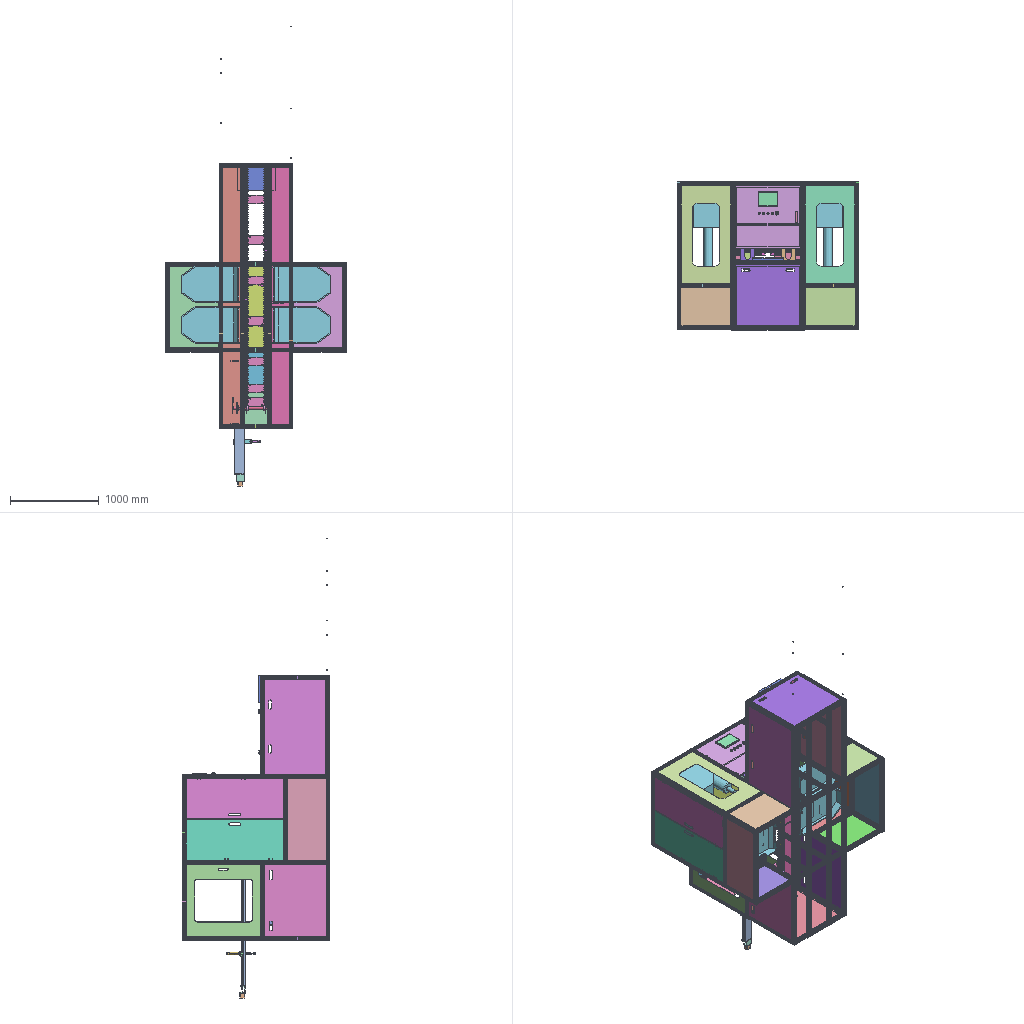Assembly | STEP file | 102 different items | 1017 placed | box 2053 x 1672 x 5196 mm
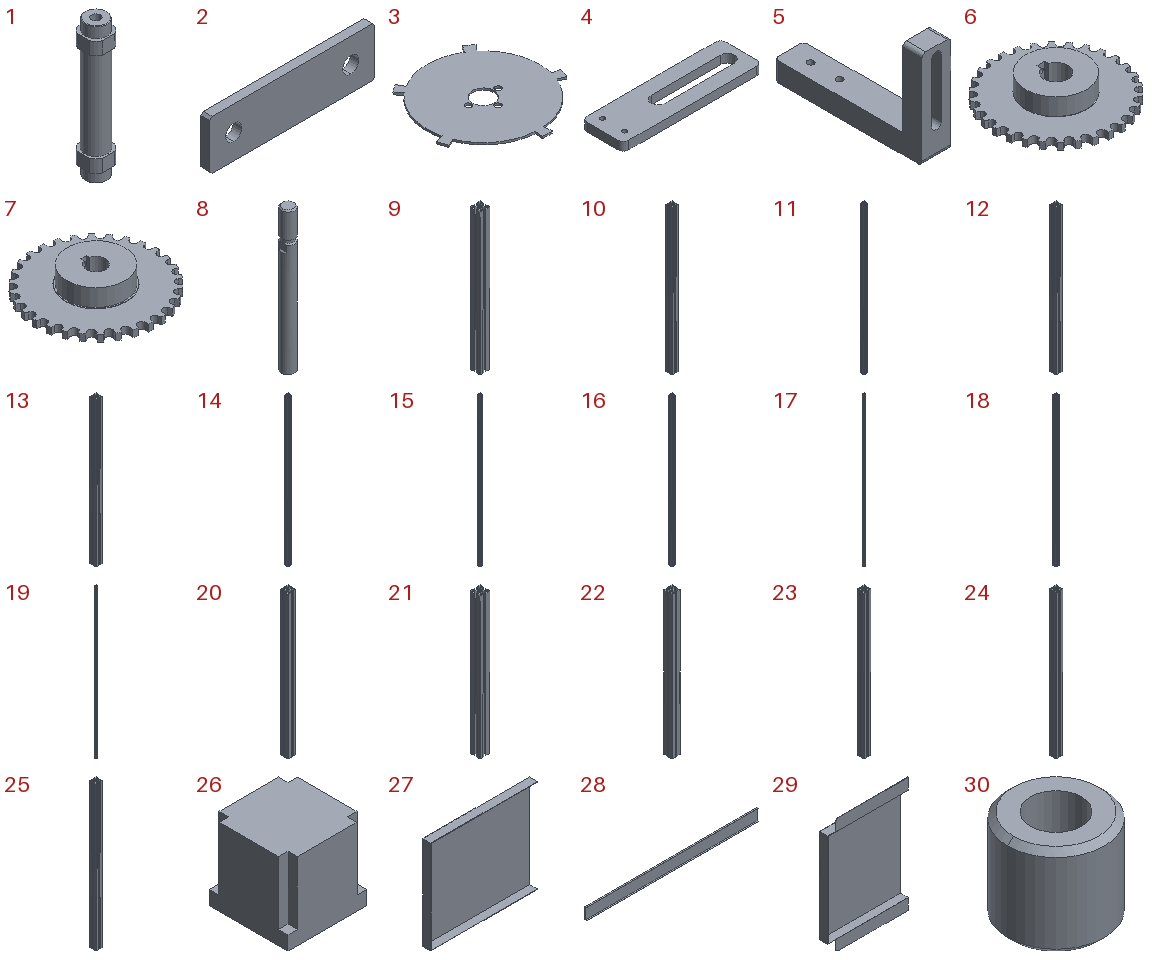Parts list (item | name | quantity | parent item | size | volume):
1 | 1-2 | x1 | in A_CM2B25-75(0)气缸-2 | 30 x 30 x 163 mm | 89864 mm3
2 | 1004-2001-0021_1004-2001-0021_1-2 | x2 | - | 134 x 7 x 40 mm | 35606 mm3
3 | 1004-2001-0084_1004-2001-0084_1-2 | x1 | - | 126.387 x 122 x 2 mm | 20227 mm3
4 | 1004-2001-0085_1004-2001-0085_1-2 | x1 | - | 50 x 15 x 3 mm | 1794 mm3
5 | 1004-2001-0086-1_1004-2001-0086-2 | x1 | - | 15 x 76 x 50 mm | 15485 mm3
6 | 1004-2001-0088_1004-2001-0088_1-2 | x2 | - | 128 x 127.688 x 25 mm | 125433 mm3
7 | 1004-2001-0089_1004-2001-0089_1-2 | x1 | - | 128 x 127.688 x 25 mm | 124903 mm3
8 | 2-2 | x1 | in A_CM2B25-75(0)气缸-2 | 10 x 10 x 108 mm | 8348 mm3
9 | 40-570-2 | x2 | in PN_0001_ASM-2 | 40 x 40 x 570 mm | 299104 mm3
10 | 40C-2 | x1 | in JZ_ASM_1_ASM-2 | 40 x 40 x 930 mm | 488011 mm3
11 | 40D-2 | x1 | in JZ_ASM_1_ASM-2 | 40 x 40 x 1670 mm | 876321 mm3
12 | 40T-2 | x1 | in JZ_ASM_1_ASM-2 | 40 x 40 x 930 mm | 488011 mm3
13 | 40U-2 | x1 | in JZ_ASM_1_ASM-2 | 40 x 40 x 930 mm | 488011 mm3
14 | 40V-2 | x1 | in JZ_ASM_1_ASM-2 | 40 x 40 x 1670 mm | 876321 mm3
15 | 40_40_1350_1-2 | x4 | in JZ_ASM_1_ASM-2 | 40 x 40 x 1970 mm | 1033744 mm3
16 | 40_40_1590_1-2 | x2 | in JZ_ASM_1_ASM-2 | 40 x 40 x 1670 mm | 876321 mm3
17 | 40_40_2730_1-2 | x2 | in JZ_ASM_1_ASM-2 | 40 x 40 x 2990 mm | 1568982 mm3
18 | 40_40_3240_1-2 | x2 | in JZ_ASM_1_ASM-2 | 40 x 40 x 1875 mm | 983893 mm3
19 | 40_40_4640_1-2 | x6 | in JZ_ASM_1_ASM-2 | 40 x 40 x 2989 mm | 1568656 mm3
20 | 40_40_470_1-2 | x2 | in JZ_ASM_1_ASM-2 | 40 x 40 x 750 mm | 393557 mm3
21 | 40_40_570-2 | x2 | in PN_0001_ASM-2 | 40 x 40 x 570 mm | 299104 mm3
22 | 40_40_700_1-2 | x14 | in JZ_ASM_1_ASM-2 | 40 x 40 x 700 mm | 367320 mm3
23 | 40_40_750_1-2 | x5 | in JZ_ASM_1_ASM-2 | 40 x 40 x 830 mm | 435537 mm3
24 | 40_40_850_1-2 | x6 | in JZ_ASM_1_ASM-2 | 40 x 40 x 850 mm | 446032 mm3
25 | 40_40_930_1-2 | x3 | in JZ_ASM_1_ASM-2 | 40 x 40 x 930 mm | 488011 mm3
26 | 57-3260步进马达-2 | x1 | in PN_0001_ASM-2 | 56 x 56 x 77.6 mm | 165142 mm3
27 | B-BAN1_1-2 | x1 | in PN_0001_ASM-2 | 400 x 30 x 350 mm | 259034 mm3
28 | B-BAN2_1-2 | x1 | in PN_0001_ASM-2 | 2950 x 30 x 200 mm | 1137225 mm3
29 | B-BAN5_1-2 | x1 | in PN_0001_ASM-2 | 300 x 30 x 430 mm | 230320 mm3
30 | CHAIN-01_1_02LT_1-2 | x220 | in TUOLIETIAO_ASM_1_ASM-2 | 8.5 x 8.5 x 8 mm | 320.312 mm3
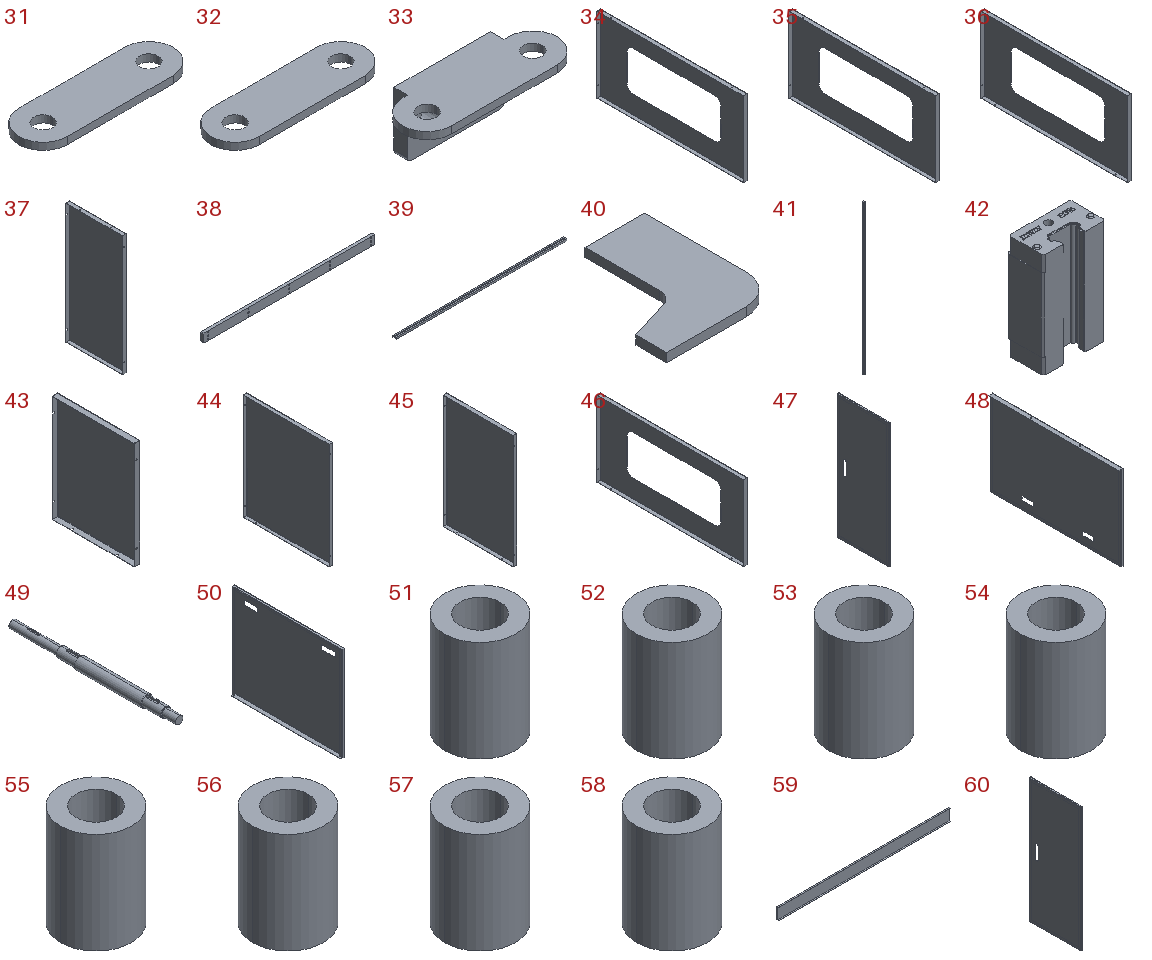31 | CHAIN-02_1_02LT_1-2 | x220 | in TUOLIETIAO_ASM_1_ASM-2 | 37.1 x 11.7 x 1.7 mm | 633.904 mm3
32 | CHAIN-03_1_02LT_1-2 | x216 | in TUOLIETIAO_ASM_1_ASM-2 | 37.1 x 11.7 x 1.7 mm | 633.904 mm3
33 | CHAIN-04_1_02LT_1-2 | x108 | in TUOLIETIAO_ASM_1_ASM-2 | 37.1 x 14.95 x 14.1 mm | 1597 mm3
34 | CHAME-2 | x1 | in PN_0001_ASM-2 | 30 x 1108 x 568 mm | 765086 mm3
35 | CHAME3-2 | x1 | in PN_0001_ASM-2 | 30 x 1108 x 568 mm | 765086 mm3
36 | CHME2-2 | x1 | in PN_0001_ASM-2 | 30 x 1108 x 568 mm | 765102 mm3
37 | CSD4-2 | x1 | in PN_0001_ASM-2 | 30 x 438 x 928 mm | 721285 mm3
38 | DAOLIECHAO-BAN_1-2 | x2 | in LIANTIAO_ASM_1_ASM-2 | 800 x 12 x 40 mm | 378698 mm3
39 | DAOLIECHAO_1-2 | x2 | in LIANTIAO_ASM_1_ASM-2 | 1861 x 40 x 20 mm | 1235153 mm3
40 | Discharge manipulator bracket.SLDASM-2 (subassembly) | x2 | in PN_0001_ASM-2 | 147.814 x 177.869 x 12 mm | 209292 mm3
41 | EG15_RAIL-2 | x1 | in EGH15CA导轨-2 | 15 x 12.5 x 1282 mm | 208724 mm3
42 | EGH15CA_BLOCK-2 | x1 | in EGH15CA导轨-2 | 34 x 19.5 x 57.8 mm | 30496 mm3
43 | FB-3_1-2 | x1 | in PN_0001_ASM-2 | 30 x 438 x 568 mm | 454976 mm3
44 | FB-6_1-2 | x1 | in PN_0001_ASM-2 | 30 x 748 x 923 mm | 1172313 mm3
45 | FB-7_1-2 | x1 | in PN_0001_ASM-2 | 30 x 568 x 923 mm | 908240 mm3
46 | FB-8_1-2 | x1 | in PN_0001_ASM-2 | 30 x 1108 x 568 mm | 765102 mm3
47 | FENGBAN-C-1_1-2 | x2 | in PN_0001_ASM-2 | 15 x 461 x 1106 mm | 897799 mm3
48 | HT-2 | x1 | in PN_0001_ASM-2 | 35 x 1080 x 702 mm | 1298798 mm3
49 | LIELUN30_1-2 | x1 | - | 30 x 432.6 x 30 mm | 218301 mm3
50 | MANIFOLD_SOLID_BREP_304524-2 | x1 | in FENBAN-1_1_ASM-2 | 30 x 816 x 696 mm | 984068 mm3
51 | MANIFOLD_SOLID_BREP_304727-2 | x1 | in FENBAN-1_1_ASM-2 | 7 x 7 x 10 mm | 259.181 mm3
52 | MANIFOLD_SOLID_BREP_304930-2 | x1 | in FENBAN-1_1_ASM-2 | 7 x 7 x 10 mm | 259.181 mm3
53 | MANIFOLD_SOLID_BREP_309818-2 | x8 | in FENBAN-2_1_ASM-2 | 7 x 7 x 10 mm | 259.181 mm3
54 | MANIFOLD_SOLID_BREP_312481-2 | x2 | in FENBAN-3_1_ASM-2 | 7 x 7 x 10 mm | 259.181 mm3
55 | MANIFOLD_SOLID_BREP_312684-2 | x2 | in FENBAN-3_1_ASM-2 | 7 x 7 x 10 mm | 259.181 mm3
56 | MANIFOLD_SOLID_BREP_315330-2 | x2 | in FENBAN-4_1_ASM-2 | 7 x 7 x 10 mm | 259.181 mm3
57 | MANIFOLD_SOLID_BREP_345006-2 | x1 | in FENBAN-5_1_ASM-2 | 7 x 7 x 10 mm | 259.181 mm3
58 | MANIFOLD_SOLID_BREP_345209-2 | x1 | in FENBAN-5_1_ASM-2 | 7 x 7 x 10 mm | 259.181 mm3
59 | MBG-2 | x1 | in PN_0001_ASM-2 | 2950 x 30 x 200 mm | 1137225 mm3
60 | ME4-2 | x1 | in PN_0001_ASM-2 | 15 x 461 x 1106 mm | 897799 mm3
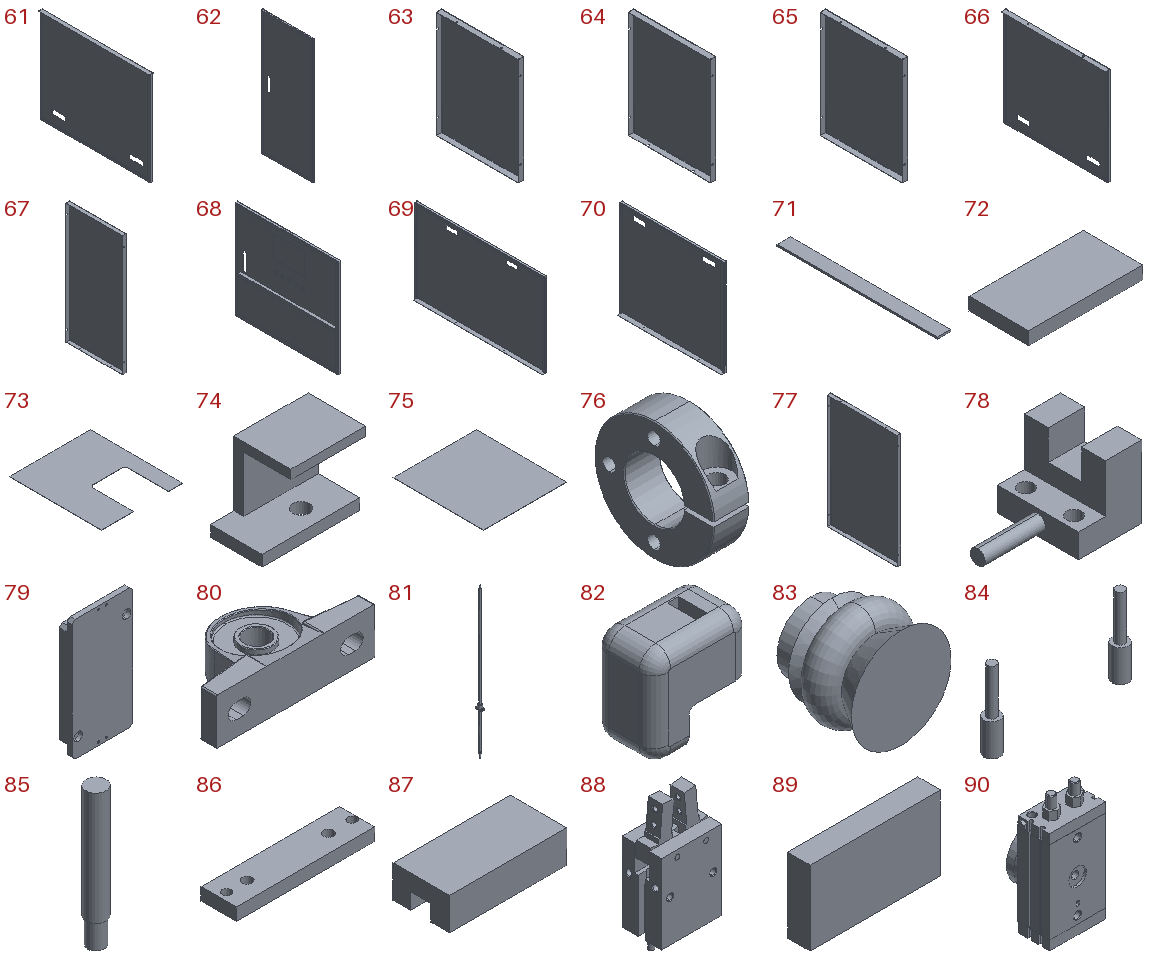61 | MEN-2 | x1 | in PN_0001_ASM-2 | 30 x 816 x 696 mm | 984067 mm3
62 | MEN5-2 | x1 | in PN_0001_ASM-2 | 15 x 461 x 1106 mm | 897799 mm3
63 | MEN7-2 | x1 | in PN_0001_ASM-2 | 30 x 438 x 568 mm | 454976 mm3
64 | MEN87-2 | x1 | in PN_0001_ASM-2 | 30 x 438 x 568 mm | 454976 mm3
65 | MENH-2 | x1 | in PN_0001_ASM-2 | 30 x 438 x 568 mm | 454976 mm3
66 | MRE-2 | x1 | in PN_0001_ASM-2 | 35 x 750 x 702 mm | 920814 mm3
67 | MSBR-1000F-2 | x1 | in PN_0001_ASM-2 | 30 x 438 x 928 mm | 721208 mm3
68 | PRT0544B-HK-005_B9T2-2 | x1 | in PN_0001_ASM-2 | 43.5 x 750 x 710 mm | 1553231 mm3
69 | PRT0544B_HI-00-2 | x1 | in PN_0001_ASM-2 | 35 x 1080 x 702 mm | 1298798 mm3
70 | PRT0544B_HI-003_B-2 | x1 | in PN_0001_ASM-2 | 35 x 750 x 702 mm | 920814 mm3
71 | Part 17 PN_0001_ASM 2 | x1 | in PN_0001_ASM-2 | 106.46 x 1282 x 15 mm | 2047522 mm3
72 | Part 19^PN_0001_ASM-2 | x1 | in PN_0001_ASM-2 | 106.46 x 56 x 12 mm | 71541 mm3
73 | Part 2 PN_0001_ASM 2 | x1 | in PN_0001_ASM-2 | 744 x 848.417 x 2 mm | 1008010 mm3
74 | Part 20 PN_0001_ASM 2 | x1 | in PN_0001_ASM-2 | 106.46 x 62.346 x 82.377 mm | 171045 mm3
75 | Part 3 PN_0001_ASM 2 | x1 | in PN_0001_ASM-2 | 751.5 x 821.5 x 2 mm | 1234714 mm3
76 | SCSTR20-12_SCSTR20-12_1-2 | x1 | - | 12 x 39.986 x 40 mm | 9883 mm3
77 | SMEB-2 | x1 | in PN_0001_ASM-2 | 30 x 568 x 923 mm | 908170 mm3
78 | - | x1 | - | 20.5 x 13.5 x 12 mm | 1060 mm3
79 | ZHIJUBAN-1_1-2 | x7 | in ZHIZHU_ASM_1_ASM-2 | 100 x 21 x 200 mm | 345878 mm3
80 | - | x2 | - | 134 x 63.85 x 39 mm | 118753 mm3
81 | r14-5b1-fsw150-2 | x1 | in PN_0001_ASM-2 | 34 x 57 x 1346 mm | 239827 mm3
82 | Product-2 | x18 | in ZHIZHU_ASM_1_ASM-2, 超升波生产线-2 | 45.9 x 28.5 x 45.9 mm | 40224 mm3
83 | 吸盘-2 | x2 | in 出料机械手-2 | 22.458 x 20 x 22.458 mm | 5536 mm3
84 | 吸盘导柱-2 | x1 | in 出料机械手-2 | 112.418 x 12.438 x 60.6 mm | 8796 mm3
85 | 导柱-2 | x16 | in 超升波生产线-2 | 12 x 12 x 83 mm | 8869 mm3
86 | 导柱Plate-2 | x1 | in 出料机械手-2 | 110.709 x 28 x 10 mm | 29224 mm3
87 | 手指夹-2 | x16 | in 超升波生产线-2 | 58 x 28 x 16 mm | 24327 mm3
88 | 手指气缸-2 | x8 | in 超升波生产线-2 | 44 x 27.6 x 88.442 mm | 60237 mm3
89 | 手指气缸座-2 | x8 | in 超升波生产线-2 | 70 x 12 x 40 mm | 33600 mm3
90 | Revolve气缸-2 | x4 | in 超升波生产线-2 | 75.4 x 57 x 152 mm | 392016 mm3
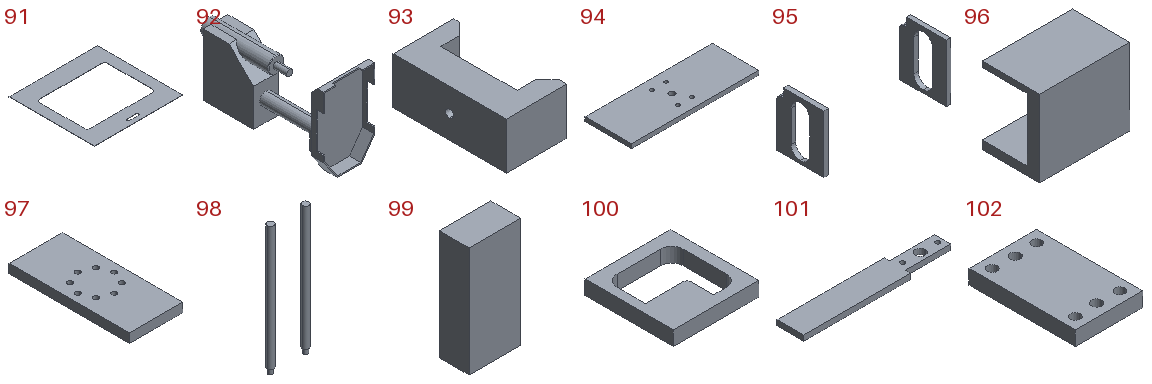91 | Plate金1-2^B9CHAO000_ASM-2 | x2 | in PN_0001_ASM-2 | 846 x 816 x 2 mm | 745734 mm3
92 | 超升坡2-2 | x4 | in 超升波生产线-2 | 415 x 1130 x 650 mm | 52548819 mm3
93 | 超声ProductFixed夹-2 | x8 | in 超升波生产线-2 | 25.961 x 48.342 x 20 mm | 16055 mm3
94 | Part 13^超升波生产线-2 | x4 | in 超升波生产线-2 | 420 x 154.525 x 14 mm | 898915 mm3
95 | Part 14^超升波生产线-2 | x4 | in 超升波生产线-2 | 420 x 154.525 x 190 mm | 580946 mm3
96 | Part 16^超升波生产线-2 | x4 | in 超升波生产线-2 | 240.448 x 154.13 x 205 mm | 2766598 mm3
97 | Part 4^超升波生产线-2 | x4 | in 超升波生产线-2 | 70 x 158 x 12 mm | 129534 mm3
98 | Part 7^出料机械手-2 | x1 | in 出料机械手-2 | 77 x 12 x 240.3 mm | 53098 mm3
99 | Part 8^出料机械手-2 | x1 | in 出料机械手-2 | 37.433 x 21.616 x 80 mm | 64732 mm3
100 | Part 95^超升波生产线-2 | x4 | in 超升波生产线-2 | 59.411 x 61.077 x 10 mm | 20947 mm3
101 | Part 9^出料机械手-2 | x1 | in 出料机械手-2 | 284.646 x 50 x 10 mm | 121671 mm3
102 | Part 9^超升波生产线-2 | x4 | in 超升波生产线-2 | 70 x 110 x 15 mm | 108190 mm3